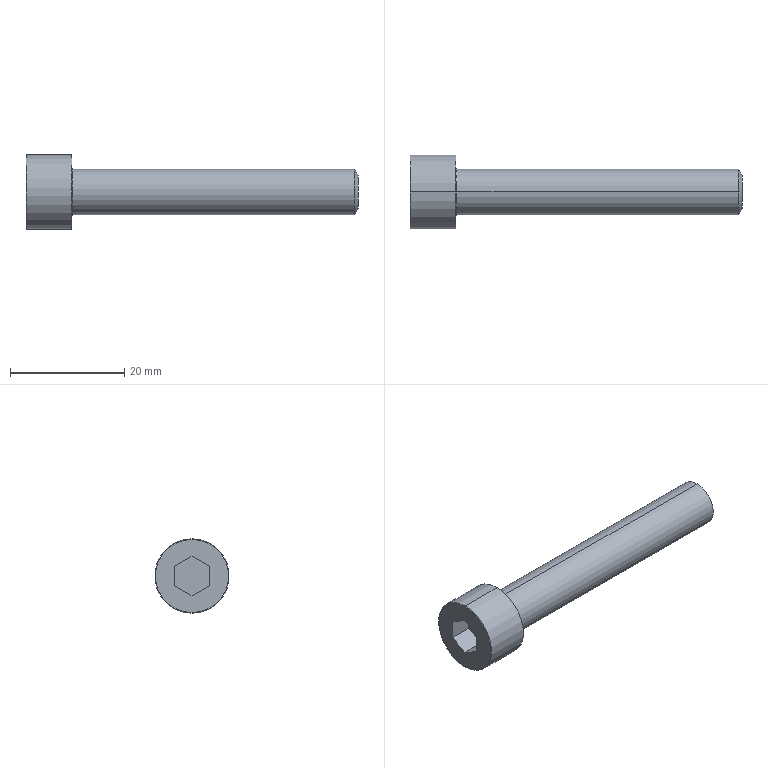Part | STEP file | 1 solid | 20 faces | box 58 x 13 x 13 mm | volume 3445 mm3 | plane 10 | torus 4 | cylinder 4 | cone 2 | commonest cylinder face diameters 8 x2 13 x2
STEP:
#1=CARTESIAN_POINT('',(0.,0.,0.));
#2=DIRECTION('',(0.,0.,1.));
#3=DIRECTION('',(1.,0.,0.));
#4=AXIS2_PLACEMENT_3D('',#1,#2,#3);
#5=CARTESIAN_POINT('',(0.,0.,6.4));
#6=VERTEX_POINT('',#5);
#7=CARTESIAN_POINT('',(0.1,0.,6.5));
#8=VERTEX_POINT('',#7);
#9=CARTESIAN_POINT('',(0.1,0.,6.4));
#10=DIRECTION('',(0.,1.,0.));
#11=DIRECTION('',(0.,0.,1.));
#12=AXIS2_PLACEMENT_3D('',#9,#10,#11);
#13=CIRCLE('',#12,0.1);
#14=CARTESIAN_POINT('',(0.1,0.,0.));
#15=DIRECTION('',(1.,0.,0.));
#16=DIRECTION('',(0.,0.,-1.));
#17=AXIS2_PLACEMENT_3D('',#14,#15,#16);
#18=TOROIDAL_SURFACE('',#17,6.4,0.1);
#19=CARTESIAN_POINT('',(3.142,0.));
#20=DIRECTION('',(0.,1.));
#21=VECTOR('',#20,1.);
#22=LINE('',#19,#21);
#23=(GEOMETRIC_REPRESENTATION_CONTEXT(2)PARAMETRIC_REPRESENTATION_CONTEXT()REPRESENTATION_CONTEXT('',''));
#24=DEFINITIONAL_REPRESENTATION('',(#22),#23);
#25=PCURVE('',#18,#24);
#26=CARTESIAN_POINT('',(0.1,0.,0.));
#27=DIRECTION('',(1.,0.,0.));
#28=DIRECTION('',(0.,0.,-1.));
#29=AXIS2_PLACEMENT_3D('',#26,#27,#28);
#30=TOROIDAL_SURFACE('',#29,6.4,0.1);
#31=CARTESIAN_POINT('',(3.142,0.));
#32=DIRECTION('',(0.,1.));
#33=VECTOR('',#32,1.);
#34=LINE('',#31,#33);
#35=(GEOMETRIC_REPRESENTATION_CONTEXT(2)PARAMETRIC_REPRESENTATION_CONTEXT()REPRESENTATION_CONTEXT('',''));
#36=DEFINITIONAL_REPRESENTATION('',(#34),#35);
#37=PCURVE('',#30,#36);
#38=SURFACE_CURVE('',#13,(#25,#37),.PCURVE_S1.);
#39=EDGE_CURVE('',#6,#8,#38,.T.);
#40=ORIENTED_EDGE('',*,*,#39,.F.);
#41=CARTESIAN_POINT('',(0.,0.,-6.4));
#42=VERTEX_POINT('',#41);
#43=CARTESIAN_POINT('',(0.,0.,0.));
#44=DIRECTION('',(-1.,0.,0.));
#45=DIRECTION('',(0.,0.,-1.));
#46=AXIS2_PLACEMENT_3D('',#43,#44,#45);
#47=CIRCLE('',#46,6.4);
#48=CARTESIAN_POINT('',(6.283,4.712));
#49=DIRECTION('',(-1.,0.));
#50=VECTOR('',#49,1.);
#51=LINE('',#48,#50);
#52=(GEOMETRIC_REPRESENTATION_CONTEXT(2)PARAMETRIC_REPRESENTATION_CONTEXT()REPRESENTATION_CONTEXT('',''));
#53=DEFINITIONAL_REPRESENTATION('',(#51),#52);
#54=PCURVE('',#18,#53);
#55=CARTESIAN_POINT('',(0.,0.,0.));
#56=DIRECTION('',(1.,0.,0.));
#57=DIRECTION('',(0.,0.,-1.));
#58=AXIS2_PLACEMENT_3D('',#55,#56,#57);
#59=PLANE('',#58);
#60=CARTESIAN_POINT('',(6.4,0.));
#61=CARTESIAN_POINT('',(6.4,-11.085));
#62=CARTESIAN_POINT('',(-3.2,-5.543));
#63=CARTESIAN_POINT('',(-12.8,0.));
#64=CARTESIAN_POINT('',(-3.2,5.543));
#65=CARTESIAN_POINT('',(6.4,11.085));
#66=CARTESIAN_POINT('',(6.4,0.));
#67=(BOUNDED_CURVE()B_SPLINE_CURVE(2,(#60,#61,#62,#63,#64,#65,#66),.UNSPECIFIED.,.T.,.F.)B_SPLINE_CURVE_WITH_KNOTS((1,2,2,2,2,1),(-2.094,0.,2.094,4.189,6.283,8.378),.UNSPECIFIED.)CURVE()GEOMETRIC_REPRESENTATION_ITEM()RATIONAL_B_SPLINE_CURVE((1.,0.5,1.,0.5,1.,0.5,1.))REPRESENTATION_ITEM(''));
#68=(GEOMETRIC_REPRESENTATION_CONTEXT(2)PARAMETRIC_REPRESENTATION_CONTEXT()REPRESENTATION_CONTEXT('',''));
#69=DEFINITIONAL_REPRESENTATION('',(#67),#68);
#70=PCURVE('',#59,#69);
#71=SURFACE_CURVE('',#47,(#54,#70),.PCURVE_S1.);
#72=EDGE_CURVE('',#42,#6,#71,.T.);
#73=ORIENTED_EDGE('',*,*,#72,.F.);
#74=CARTESIAN_POINT('',(0.1,0.,-6.5));
#75=VERTEX_POINT('',#74);
#76=CARTESIAN_POINT('',(0.1,0.,-6.4));
#77=DIRECTION('',(0.,-1.,0.));
#78=DIRECTION('',(0.,0.,-1.));
#79=AXIS2_PLACEMENT_3D('',#76,#77,#78);
#80=CIRCLE('',#79,0.1);
#81=CARTESIAN_POINT('',(6.283,0.));
#82=DIRECTION('',(0.,1.));
#83=VECTOR('',#82,1.);
#84=LINE('',#81,#83);
#85=(GEOMETRIC_REPRESENTATION_CONTEXT(2)PARAMETRIC_REPRESENTATION_CONTEXT()REPRESENTATION_CONTEXT('',''));
#86=DEFINITIONAL_REPRESENTATION('',(#84),#85);
#87=PCURVE('',#18,#86);
#88=CARTESIAN_POINT('',(0.,0.));
#89=DIRECTION('',(0.,1.));
#90=VECTOR('',#89,1.);
#91=LINE('',#88,#90);
#92=(GEOMETRIC_REPRESENTATION_CONTEXT(2)PARAMETRIC_REPRESENTATION_CONTEXT()REPRESENTATION_CONTEXT('',''));
#93=DEFINITIONAL_REPRESENTATION('',(#91),#92);
#94=PCURVE('',#30,#93);
#95=SURFACE_CURVE('',#80,(#87,#94),.PCURVE_S1.);
#96=EDGE_CURVE('',#42,#75,#95,.T.);
#97=ORIENTED_EDGE('',*,*,#96,.T.);
#98=CARTESIAN_POINT('',(0.1,0.,0.));
#99=DIRECTION('',(1.,0.,0.));
#100=DIRECTION('',(0.,0.,-1.));
#101=AXIS2_PLACEMENT_3D('',#98,#99,#100);
#102=CIRCLE('',#101,6.5);
#103=CARTESIAN_POINT('',(0.,6.283));
#104=DIRECTION('',(1.,0.));
#105=VECTOR('',#104,1.);
#106=LINE('',#103,#105);
#107=(GEOMETRIC_REPRESENTATION_CONTEXT(2)PARAMETRIC_REPRESENTATION_CONTEXT()REPRESENTATION_CONTEXT('',''));
#108=DEFINITIONAL_REPRESENTATION('',(#106),#107);
#109=PCURVE('',#18,#108);
#110=CARTESIAN_POINT('',(0.,0.,0.));
#111=DIRECTION('',(-1.,0.,0.));
#112=DIRECTION('',(0.,0.,1.));
#113=AXIS2_PLACEMENT_3D('',#110,#111,#112);
#114=CYLINDRICAL_SURFACE('',#113,6.5);
#115=CARTESIAN_POINT('',(9.425,-0.1));
#116=DIRECTION('',(-1.,0.));
#117=VECTOR('',#116,1.);
#118=LINE('',#115,#117);
#119=(GEOMETRIC_REPRESENTATION_CONTEXT(2)PARAMETRIC_REPRESENTATION_CONTEXT()REPRESENTATION_CONTEXT('',''));
#120=DEFINITIONAL_REPRESENTATION('',(#118),#119);
#121=PCURVE('',#114,#120);
#122=SURFACE_CURVE('',#102,(#109,#121),.PCURVE_S1.);
#123=EDGE_CURVE('',#8,#75,#122,.T.);
#124=ORIENTED_EDGE('',*,*,#123,.F.);
#125=EDGE_LOOP('',(#40,#73,#97,#124));
#126=FACE_BOUND('',#125,.T.);
#127=ADVANCED_FACE('',(#126),#18,.T.);
#128=CARTESIAN_POINT('',(58.,0.,2.917));
#129=VERTEX_POINT('',#128);
#130=CARTESIAN_POINT('',(58.,0.,-2.917));
#131=VERTEX_POINT('',#130);
#132=CARTESIAN_POINT('',(58.,0.,0.));
#133=DIRECTION('',(-1.,0.,0.));
#134=DIRECTION('',(0.,0.,1.));
#135=AXIS2_PLACEMENT_3D('',#132,#133,#134);
#136=CIRCLE('',#135,2.917);
#137=CARTESIAN_POINT('',(58.,4.,0.));
#138=DIRECTION('',(-1.,0.,0.));
#139=DIRECTION('',(0.,0.,1.));
#140=AXIS2_PLACEMENT_3D('',#137,#138,#139);
#141=PLANE('',#140);
#142=CARTESIAN_POINT('',(0.,-4.));
#143=DIRECTION('',(1.,0.));
#144=AXIS2_PLACEMENT_2D('',#142,#143);
#145=CIRCLE('',#144,2.917);
#146=(GEOMETRIC_REPRESENTATION_CONTEXT(2)PARAMETRIC_REPRESENTATION_CONTEXT()REPRESENTATION_CONTEXT('',''));
#147=DEFINITIONAL_REPRESENTATION('',(#145),#146);
#148=PCURVE('',#141,#147);
#149=CARTESIAN_POINT('',(57.375,0.,0.));
#150=DIRECTION('',(-1.,0.,0.));
#151=DIRECTION('',(0.,0.,1.));
#152=AXIS2_PLACEMENT_3D('',#149,#150,#151);
#153=CONICAL_SURFACE('',#152,4.,1.047);
#154=CARTESIAN_POINT('',(0.,-0.625));
#155=DIRECTION('',(1.,0.));
#156=VECTOR('',#155,1.);
#157=LINE('',#154,#156);
#158=(GEOMETRIC_REPRESENTATION_CONTEXT(2)PARAMETRIC_REPRESENTATION_CONTEXT()REPRESENTATION_CONTEXT('',''));
#159=DEFINITIONAL_REPRESENTATION('',(#157),#158);
#160=PCURVE('',#153,#159);
#161=SURFACE_CURVE('',#136,(#148,#160),.PCURVE_S1.);
#162=EDGE_CURVE('',#129,#131,#161,.T.);
#163=ORIENTED_EDGE('',*,*,#162,.F.);
#164=CARTESIAN_POINT('',(58.,0.,0.));
#165=DIRECTION('',(-1.,0.,0.));
#166=DIRECTION('',(0.,0.,1.));
#167=AXIS2_PLACEMENT_3D('',#164,#165,#166);
#168=CIRCLE('',#167,2.917);
#169=CARTESIAN_POINT('',(0.,-4.));
#170=DIRECTION('',(1.,0.));
#171=AXIS2_PLACEMENT_2D('',#169,#170);
#172=CIRCLE('',#171,2.917);
#173=(GEOMETRIC_REPRESENTATION_CONTEXT(2)PARAMETRIC_REPRESENTATION_CONTEXT()REPRESENTATION_CONTEXT('',''));
#174=DEFINITIONAL_REPRESENTATION('',(#172),#173);
#175=PCURVE('',#141,#174);
#176=CARTESIAN_POINT('',(57.375,0.,0.));
#177=DIRECTION('',(-1.,0.,0.));
#178=DIRECTION('',(0.,0.,1.));
#179=AXIS2_PLACEMENT_3D('',#176,#177,#178);
#180=CONICAL_SURFACE('',#179,4.,1.047);
#181=CARTESIAN_POINT('',(0.,-0.625));
#182=DIRECTION('',(1.,0.));
#183=VECTOR('',#182,1.);
#184=LINE('',#181,#183);
#185=(GEOMETRIC_REPRESENTATION_CONTEXT(2)PARAMETRIC_REPRESENTATION_CONTEXT()REPRESENTATION_CONTEXT('',''));
#186=DEFINITIONAL_REPRESENTATION('',(#184),#185);
#187=PCURVE('',#180,#186);
#188=SURFACE_CURVE('',#168,(#175,#187),.PCURVE_S1.);
#189=EDGE_CURVE('',#131,#129,#188,.T.);
#190=ORIENTED_EDGE('',*,*,#189,.F.);
#191=EDGE_LOOP('',(#163,#190));
#192=FACE_BOUND('',#191,.T.);
#193=ADVANCED_FACE('',(#192),#141,.F.);
#194=CARTESIAN_POINT('',(57.375,0.,-4.));
#195=VERTEX_POINT('',#194);
#196=CARTESIAN_POINT('',(57.375,0.,-4.));
#197=DIRECTION('',(-0.5,0.,-0.866));
#198=VECTOR('',#197,1.);
#199=LINE('',#196,#198);
#200=CARTESIAN_POINT('',(3.142,0.));
#201=DIRECTION('',(0.,1.));
#202=VECTOR('',#201,1.);
#203=LINE('',#200,#202);
#204=(GEOMETRIC_REPRESENTATION_CONTEXT(2)PARAMETRIC_REPRESENTATION_CONTEXT()REPRESENTATION_CONTEXT('',''));
#205=DEFINITIONAL_REPRESENTATION('',(#203),#204);
#206=PCURVE('',#180,#205);
#207=CARTESIAN_POINT('',(3.142,0.));
#208=DIRECTION('',(0.,1.));
#209=VECTOR('',#208,1.);
#210=LINE('',#207,#209);
#211=(GEOMETRIC_REPRESENTATION_CONTEXT(2)PARAMETRIC_REPRESENTATION_CONTEXT()REPRESENTATION_CONTEXT('',''));
#212=DEFINITIONAL_REPRESENTATION('',(#210),#211);
#213=PCURVE('',#153,#212);
#214=SURFACE_CURVE('',#199,(#206,#213),.PCURVE_S1.);
#215=EDGE_CURVE('',#131,#195,#214,.T.);
#216=ORIENTED_EDGE('',*,*,#215,.F.);
#217=ORIENTED_EDGE('',*,*,#189,.T.);
#218=CARTESIAN_POINT('',(57.375,0.,4.));
#219=VERTEX_POINT('',#218);
#220=CARTESIAN_POINT('',(57.375,0.,4.));
#221=DIRECTION('',(-0.5,0.,0.866));
#222=VECTOR('',#221,1.);
#223=LINE('',#220,#222);
#224=CARTESIAN_POINT('',(6.283,0.));
#225=DIRECTION('',(0.,1.));
#226=VECTOR('',#225,1.);
#227=LINE('',#224,#226);
#228=(GEOMETRIC_REPRESENTATION_CONTEXT(2)PARAMETRIC_REPRESENTATION_CONTEXT()REPRESENTATION_CONTEXT('',''));
#229=DEFINITIONAL_REPRESENTATION('',(#227),#228);
#230=PCURVE('',#180,#229);
#231=CARTESIAN_POINT('',(0.,0.));
#232=DIRECTION('',(0.,1.));
#233=VECTOR('',#232,1.);
#234=LINE('',#231,#233);
#235=(GEOMETRIC_REPRESENTATION_CONTEXT(2)PARAMETRIC_REPRESENTATION_CONTEXT()REPRESENTATION_CONTEXT('',''));
#236=DEFINITIONAL_REPRESENTATION('',(#234),#235);
#237=PCURVE('',#153,#236);
#238=SURFACE_CURVE('',#223,(#230,#237),.PCURVE_S1.);
#239=EDGE_CURVE('',#129,#219,#238,.T.);
#240=ORIENTED_EDGE('',*,*,#239,.T.);
#241=CARTESIAN_POINT('',(57.375,0.,0.));
#242=DIRECTION('',(-1.,0.,0.));
#243=DIRECTION('',(0.,0.,1.));
#244=AXIS2_PLACEMENT_3D('',#241,#242,#243);
#245=CIRCLE('',#244,4.);
#246=CARTESIAN_POINT('',(0.,0.));
#247=DIRECTION('',(1.,0.));
#248=VECTOR('',#247,1.);
#249=LINE('',#246,#248);
#250=(GEOMETRIC_REPRESENTATION_CONTEXT(2)PARAMETRIC_REPRESENTATION_CONTEXT()REPRESENTATION_CONTEXT('',''));
#251=DEFINITIONAL_REPRESENTATION('',(#249),#250);
#252=PCURVE('',#180,#251);
#253=CARTESIAN_POINT('',(0.,0.,0.));
#254=DIRECTION('',(-1.,0.,0.));
#255=DIRECTION('',(0.,0.,1.));
#256=AXIS2_PLACEMENT_3D('',#253,#254,#255);
#257=CYLINDRICAL_SURFACE('',#256,4.);
#258=CARTESIAN_POINT('',(0.,-57.375));
#259=DIRECTION('',(1.,0.));
#260=VECTOR('',#259,1.);
#261=LINE('',#258,#260);
#262=(GEOMETRIC_REPRESENTATION_CONTEXT(2)PARAMETRIC_REPRESENTATION_CONTEXT()REPRESENTATION_CONTEXT('',''));
#263=DEFINITIONAL_REPRESENTATION('',(#261),#262);
#264=PCURVE('',#257,#263);
#265=SURFACE_CURVE('',#245,(#252,#264),.PCURVE_S1.);
#266=EDGE_CURVE('',#195,#219,#265,.T.);
#267=ORIENTED_EDGE('',*,*,#266,.F.);
#268=EDGE_LOOP('',(#216,#217,#240,#267));
#269=FACE_BOUND('',#268,.T.);
#270=ADVANCED_FACE('',(#269),#180,.T.);
#271=CARTESIAN_POINT('',(4.,-2.97,1.715));
#272=VERTEX_POINT('',#271);
#273=CARTESIAN_POINT('',(4.,0.,3.43));
#274=VERTEX_POINT('',#273);
#275=CARTESIAN_POINT('',(4.,-2.97,1.715));
#276=DIRECTION('',(0.,0.866,0.5));
#277=VECTOR('',#276,1.);
#278=LINE('',#275,#277);
#279=CARTESIAN_POINT('',(4.,-2.97,1.715));
#280=DIRECTION('',(1.,0.,0.));
#281=DIRECTION('',(0.,0.,-1.));
#282=AXIS2_PLACEMENT_3D('',#279,#280,#281);
#283=PLANE('',#282);
#284=CARTESIAN_POINT('',(0.,0.));
#285=DIRECTION('',(-0.5,0.866));
#286=VECTOR('',#285,1.);
#287=LINE('',#284,#286);
#288=(GEOMETRIC_REPRESENTATION_CONTEXT(2)PARAMETRIC_REPRESENTATION_CONTEXT()REPRESENTATION_CONTEXT('',''));
#289=DEFINITIONAL_REPRESENTATION('',(#287),#288);
#290=PCURVE('',#283,#289);
#291=CARTESIAN_POINT('',(4.,-2.97,1.715));
#292=DIRECTION('',(0.,-0.5,0.866));
#293=DIRECTION('',(0.,-0.866,-0.5));
#294=AXIS2_PLACEMENT_3D('',#291,#292,#293);
#295=PLANE('',#294);
#296=CARTESIAN_POINT('',(0.,0.));
#297=DIRECTION('',(-1.,0.));
#298=VECTOR('',#297,1.);
#299=LINE('',#296,#298);
#300=(GEOMETRIC_REPRESENTATION_CONTEXT(2)PARAMETRIC_REPRESENTATION_CONTEXT()REPRESENTATION_CONTEXT('',''));
#301=DEFINITIONAL_REPRESENTATION('',(#299),#300);
#302=PCURVE('',#295,#301);
#303=SURFACE_CURVE('',#278,(#290,#302),.PCURVE_S1.);
#304=EDGE_CURVE('',#272,#274,#303,.T.);
#305=ORIENTED_EDGE('',*,*,#304,.T.);
#306=CARTESIAN_POINT('',(4.,2.97,1.715));
#307=VERTEX_POINT('',#306);
#308=CARTESIAN_POINT('',(4.,0.,3.43));
#309=DIRECTION('',(0.,0.866,-0.5));
#310=VECTOR('',#309,1.);
#311=LINE('',#308,#310);
#312=CARTESIAN_POINT('',(-1.715,2.97));
#313=DIRECTION('',(0.5,0.866));
#314=VECTOR('',#313,1.);
#315=LINE('',#312,#314);
#316=(GEOMETRIC_REPRESENTATION_CONTEXT(2)PARAMETRIC_REPRESENTATION_CONTEXT()REPRESENTATION_CONTEXT('',''));
#317=DEFINITIONAL_REPRESENTATION('',(#315),#316);
#318=PCURVE('',#283,#317);
#319=CARTESIAN_POINT('',(4.,0.,3.43));
#320=DIRECTION('',(0.,0.5,0.866));
#321=DIRECTION('',(0.,-0.866,0.5));
#322=AXIS2_PLACEMENT_3D('',#319,#320,#321);
#323=PLANE('',#322);
#324=CARTESIAN_POINT('',(0.,0.));
#325=DIRECTION('',(-1.,0.));
#326=VECTOR('',#325,1.);
#327=LINE('',#324,#326);
#328=(GEOMETRIC_REPRESENTATION_CONTEXT(2)PARAMETRIC_REPRESENTATION_CONTEXT()REPRESENTATION_CONTEXT('',''));
#329=DEFINITIONAL_REPRESENTATION('',(#327),#328);
#330=PCURVE('',#323,#329);
#331=SURFACE_CURVE('',#311,(#318,#330),.PCURVE_S1.);
#332=EDGE_CURVE('',#274,#307,#331,.T.);
#333=ORIENTED_EDGE('',*,*,#332,.T.);
#334=CARTESIAN_POINT('',(4.,2.97,-1.715));
#335=VERTEX_POINT('',#334);
#336=CARTESIAN_POINT('',(4.,2.97,1.715));
#337=DIRECTION('',(0.,0.,-1.));
#338=VECTOR('',#337,1.);
#339=LINE('',#336,#338);
#340=CARTESIAN_POINT('',(0.,5.941));
#341=DIRECTION('',(1.,0.));
#342=VECTOR('',#341,1.);
#343=LINE('',#340,#342);
#344=(GEOMETRIC_REPRESENTATION_CONTEXT(2)PARAMETRIC_REPRESENTATION_CONTEXT()REPRESENTATION_CONTEXT('',''));
#345=DEFINITIONAL_REPRESENTATION('',(#343),#344);
#346=PCURVE('',#283,#345);
#347=CARTESIAN_POINT('',(4.,2.97,1.715));
#348=DIRECTION('',(0.,1.,0.));
#349=DIRECTION('',(0.,0.,1.));
#350=AXIS2_PLACEMENT_3D('',#347,#348,#349);
#351=PLANE('',#350);
#352=CARTESIAN_POINT('',(0.,0.));
#353=DIRECTION('',(-1.,0.));
#354=VECTOR('',#353,1.);
#355=LINE('',#352,#354);
#356=(GEOMETRIC_REPRESENTATION_CONTEXT(2)PARAMETRIC_REPRESENTATION_CONTEXT()REPRESENTATION_CONTEXT('',''));
#357=DEFINITIONAL_REPRESENTATION('',(#355),#356);
#358=PCURVE('',#351,#357);
#359=SURFACE_CURVE('',#339,(#346,#358),.PCURVE_S1.);
#360=EDGE_CURVE('',#307,#335,#359,.T.);
#361=ORIENTED_EDGE('',*,*,#360,.T.);
#362=CARTESIAN_POINT('',(4.,0.,-3.43));
#363=VERTEX_POINT('',#362);
#364=CARTESIAN_POINT('',(4.,2.97,-1.715));
#365=DIRECTION('',(0.,-0.866,-0.5));
#366=VECTOR('',#365,1.);
#367=LINE('',#364,#366);
#368=CARTESIAN_POINT('',(3.43,5.941));
#369=DIRECTION('',(0.5,-0.866));
#370=VECTOR('',#369,1.);
#371=LINE('',#368,#370);
#372=(GEOMETRIC_REPRESENTATION_CONTEXT(2)PARAMETRIC_REPRESENTATION_CONTEXT()REPRESENTATION_CONTEXT('',''));
#373=DEFINITIONAL_REPRESENTATION('',(#371),#372);
#374=PCURVE('',#283,#373);
#375=CARTESIAN_POINT('',(4.,2.97,-1.715));
#376=DIRECTION('',(0.,0.5,-0.866));
#377=DIRECTION('',(0.,0.866,0.5));
#378=AXIS2_PLACEMENT_3D('',#375,#376,#377);
#379=PLANE('',#378);
#380=CARTESIAN_POINT('',(0.,0.));
#381=DIRECTION('',(-1.,0.));
#382=VECTOR('',#381,1.);
#383=LINE('',#380,#382);
#384=(GEOMETRIC_REPRESENTATION_CONTEXT(2)PARAMETRIC_REPRESENTATION_CONTEXT()REPRESENTATION_CONTEXT('',''));
#385=DEFINITIONAL_REPRESENTATION('',(#383),#384);
#386=PCURVE('',#379,#385);
#387=SURFACE_CURVE('',#367,(#374,#386),.PCURVE_S1.);
#388=EDGE_CURVE('',#335,#363,#387,.T.);
#389=ORIENTED_EDGE('',*,*,#388,.T.);
#390=CARTESIAN_POINT('',(4.,-2.97,-1.715));
#391=VERTEX_POINT('',#390);
#392=CARTESIAN_POINT('',(4.,0.,-3.43));
#393=DIRECTION('',(0.,-0.866,0.5));
#394=VECTOR('',#393,1.);
#395=LINE('',#392,#394);
#396=CARTESIAN_POINT('',(5.145,2.97));
#397=DIRECTION('',(-0.5,-0.866));
#398=VECTOR('',#397,1.);
#399=LINE('',#396,#398);
#400=(GEOMETRIC_REPRESENTATION_CONTEXT(2)PARAMETRIC_REPRESENTATION_CONTEXT()REPRESENTATION_CONTEXT('',''));
#401=DEFINITIONAL_REPRESENTATION('',(#399),#400);
#402=PCURVE('',#283,#401);
#403=CARTESIAN_POINT('',(4.,0.,-3.43));
#404=DIRECTION('',(0.,-0.5,-0.866));
#405=DIRECTION('',(0.,0.866,-0.5));
#406=AXIS2_PLACEMENT_3D('',#403,#404,#405);
#407=PLANE('',#406);
#408=CARTESIAN_POINT('',(0.,0.));
#409=DIRECTION('',(-1.,0.));
#410=VECTOR('',#409,1.);
#411=LINE('',#408,#410);
#412=(GEOMETRIC_REPRESENTATION_CONTEXT(2)PARAMETRIC_REPRESENTATION_CONTEXT()REPRESENTATION_CONTEXT('',''));
#413=DEFINITIONAL_REPRESENTATION('',(#411),#412);
#414=PCURVE('',#407,#413);
#415=SURFACE_CURVE('',#395,(#402,#414),.PCURVE_S1.);
#416=EDGE_CURVE('',#363,#391,#415,.T.);
#417=ORIENTED_EDGE('',*,*,#416,.T.);
#418=CARTESIAN_POINT('',(4.,-2.97,-1.715));
#419=DIRECTION('',(0.,0.,1.));
#420=VECTOR('',#419,1.);
#421=LINE('',#418,#420);
#422=CARTESIAN_POINT('',(3.43,0.));
#423=DIRECTION('',(-1.,0.));
#424=VECTOR('',#423,1.);
#425=LINE('',#422,#424);
#426=(GEOMETRIC_REPRESENTATION_CONTEXT(2)PARAMETRIC_REPRESENTATION_CONTEXT()REPRESENTATION_CONTEXT('',''));
#427=DEFINITIONAL_REPRESENTATION('',(#425),#426);
#428=PCURVE('',#283,#427);
#429=CARTESIAN_POINT('',(4.,-2.97,-1.715));
#430=DIRECTION('',(0.,-1.,0.));
#431=DIRECTION('',(0.,0.,-1.));
#432=AXIS2_PLACEMENT_3D('',#429,#430,#431);
#433=PLANE('',#432);
#434=CARTESIAN_POINT('',(0.,0.));
#435=DIRECTION('',(-1.,0.));
#436=VECTOR('',#435,1.);
#437=LINE('',#434,#436);
#438=(GEOMETRIC_REPRESENTATION_CONTEXT(2)PARAMETRIC_REPRESENTATION_CONTEXT()REPRESENTATION_CONTEXT('',''));
#439=DEFINITIONAL_REPRESENTATION('',(#437),#438);
#440=PCURVE('',#433,#439);
#441=SURFACE_CURVE('',#421,(#428,#440),.PCURVE_S1.);
#442=EDGE_CURVE('',#391,#272,#441,.T.);
#443=ORIENTED_EDGE('',*,*,#442,.T.);
#444=EDGE_LOOP('',(#305,#333,#361,#389,#417,#443));
#445=FACE_BOUND('',#444,.T.);
#446=ADVANCED_FACE('',(#445),#283,.F.);
#447=CARTESIAN_POINT('',(0.,0.,3.43));
#448=VERTEX_POINT('',#447);
#449=CARTESIAN_POINT('',(0.,2.97,1.715));
#450=VERTEX_POINT('',#449);
#451=CARTESIAN_POINT('',(0.,0.,3.43));
#452=DIRECTION('',(0.,0.866,-0.5));
#453=VECTOR('',#452,1.);
#454=LINE('',#451,#453);
#455=CARTESIAN_POINT('',(0.,-4.));
#456=DIRECTION('',(-1.,0.));
#457=VECTOR('',#456,1.);
#458=LINE('',#455,#457);
#459=(GEOMETRIC_REPRESENTATION_CONTEXT(2)PARAMETRIC_REPRESENTATION_CONTEXT()REPRESENTATION_CONTEXT('',''));
#460=DEFINITIONAL_REPRESENTATION('',(#458),#459);
#461=PCURVE('',#323,#460);
#462=CARTESIAN_POINT('',(-3.43,0.));
#463=DIRECTION('',(0.5,0.866));
#464=VECTOR('',#463,1.);
#465=LINE('',#462,#464);
#466=(GEOMETRIC_REPRESENTATION_CONTEXT(2)PARAMETRIC_REPRESENTATION_CONTEXT()REPRESENTATION_CONTEXT('',''));
#467=DEFINITIONAL_REPRESENTATION('',(#465),#466);
#468=PCURVE('',#59,#467);
#469=SURFACE_CURVE('',#454,(#461,#468),.PCURVE_S1.);
#470=EDGE_CURVE('',#448,#450,#469,.T.);
#471=ORIENTED_EDGE('',*,*,#470,.T.);
#472=CARTESIAN_POINT('',(4.,2.97,1.715));
#473=DIRECTION('',(-1.,0.,0.));
#474=VECTOR('',#473,1.);
#475=LINE('',#472,#474);
#476=CARTESIAN_POINT('',(-3.43,0.));
#477=DIRECTION('',(0.,-1.));
#478=VECTOR('',#477,1.);
#479=LINE('',#476,#478);
#480=(GEOMETRIC_REPRESENTATION_CONTEXT(2)PARAMETRIC_REPRESENTATION_CONTEXT()REPRESENTATION_CONTEXT('',''));
#481=DEFINITIONAL_REPRESENTATION('',(#479),#480);
#482=PCURVE('',#323,#481);
#483=CARTESIAN_POINT('',(0.,0.));
#484=DIRECTION('',(0.,-1.));
#485=VECTOR('',#484,1.);
#486=LINE('',#483,#485);
#487=(GEOMETRIC_REPRESENTATION_CONTEXT(2)PARAMETRIC_REPRESENTATION_CONTEXT()REPRESENTATION_CONTEXT('',''));
#488=DEFINITIONAL_REPRESENTATION('',(#486),#487);
#489=PCURVE('',#351,#488);
#490=SURFACE_CURVE('',#475,(#482,#489),.PCURVE_S1.);
#491=EDGE_CURVE('',#307,#450,#490,.T.);
#492=ORIENTED_EDGE('',*,*,#491,.F.);
#493=ORIENTED_EDGE('',*,*,#332,.F.);
#494=CARTESIAN_POINT('',(4.,0.,3.43));
#495=DIRECTION('',(-1.,0.,0.));
#496=VECTOR('',#495,1.);
#497=LINE('',#494,#496);
#498=CARTESIAN_POINT('',(0.,0.));
#499=DIRECTION('',(0.,-1.));
#500=VECTOR('',#499,1.);
#501=LINE('',#498,#500);
#502=(GEOMETRIC_REPRESENTATION_CONTEXT(2)PARAMETRIC_REPRESENTATION_CONTEXT()REPRESENTATION_CONTEXT('',''));
#503=DEFINITIONAL_REPRESENTATION('',(#501),#502);
#504=PCURVE('',#323,#503);
#505=CARTESIAN_POINT('',(-3.43,0.));
#506=DIRECTION('',(0.,-1.));
#507=VECTOR('',#506,1.);
#508=LINE('',#505,#507);
#509=(GEOMETRIC_REPRESENTATION_CONTEXT(2)PARAMETRIC_REPRESENTATION_CONTEXT()REPRESENTATION_CONTEXT('',''));
#510=DEFINITIONAL_REPRESENTATION('',(#508),#509);
#511=PCURVE('',#295,#510);
#512=SURFACE_CURVE('',#497,(#504,#511),.PCURVE_S1.);
#513=EDGE_CURVE('',#274,#448,#512,.T.);
#514=ORIENTED_EDGE('',*,*,#513,.T.);
#515=EDGE_LOOP('',(#471,#492,#493,#514));
#516=FACE_BOUND('',#515,.T.);
#517=ADVANCED_FACE('',(#516),#323,.F.);
#518=CARTESIAN_POINT('',(0.,2.97,-1.715));
#519=VERTEX_POINT('',#518);
#520=CARTESIAN_POINT('',(0.,2.97,1.715));
#521=DIRECTION('',(0.,0.,-1.));
#522=VECTOR('',#521,1.);
#523=LINE('',#520,#522);
#524=CARTESIAN_POINT('',(0.,-4.));
#525=DIRECTION('',(-1.,0.));
#526=VECTOR('',#525,1.);
#527=LINE('',#524,#526);
#528=(GEOMETRIC_REPRESENTATION_CONTEXT(2)PARAMETRIC_REPRESENTATION_CONTEXT()REPRESENTATION_CONTEXT('',''));
#529=DEFINITIONAL_REPRESENTATION('',(#527),#528);
#530=PCURVE('',#351,#529);
#531=CARTESIAN_POINT('',(-1.715,2.97));
#532=DIRECTION('',(1.,0.));
#533=VECTOR('',#532,1.);
#534=LINE('',#531,#533);
#535=(GEOMETRIC_REPRESENTATION_CONTEXT(2)PARAMETRIC_REPRESENTATION_CONTEXT()REPRESENTATION_CONTEXT('',''));
#536=DEFINITIONAL_REPRESENTATION('',(#534),#535);
#537=PCURVE('',#59,#536);
#538=SURFACE_CURVE('',#523,(#530,#537),.PCURVE_S1.);
#539=EDGE_CURVE('',#450,#519,#538,.T.);
#540=ORIENTED_EDGE('',*,*,#539,.T.);
#541=CARTESIAN_POINT('',(4.,2.97,-1.715));
#542=DIRECTION('',(-1.,0.,0.));
#543=VECTOR('',#542,1.);
#544=LINE('',#541,#543);
#545=CARTESIAN_POINT('',(-3.43,0.));
#546=DIRECTION('',(0.,-1.));
#547=VECTOR('',#546,1.);
#548=LINE('',#545,#547);
#549=(GEOMETRIC_REPRESENTATION_CONTEXT(2)PARAMETRIC_REPRESENTATION_CONTEXT()REPRESENTATION_CONTEXT('',''));
#550=DEFINITIONAL_REPRESENTATION('',(#548),#549);
#551=PCURVE('',#351,#550);
#552=CARTESIAN_POINT('',(0.,0.));
#553=DIRECTION('',(0.,-1.));
#554=VECTOR('',#553,1.);
#555=LINE('',#552,#554);
#556=(GEOMETRIC_REPRESENTATION_CONTEXT(2)PARAMETRIC_REPRESENTATION_CONTEXT()REPRESENTATION_CONTEXT('',''));
#557=DEFINITIONAL_REPRESENTATION('',(#555),#556);
#558=PCURVE('',#379,#557);
#559=SURFACE_CURVE('',#544,(#551,#558),.PCURVE_S1.);
#560=EDGE_CURVE('',#335,#519,#559,.T.);
#561=ORIENTED_EDGE('',*,*,#560,.F.);
#562=ORIENTED_EDGE('',*,*,#360,.F.);
#563=ORIENTED_EDGE('',*,*,#491,.T.);
#564=EDGE_LOOP('',(#540,#561,#562,#563));
#565=FACE_BOUND('',#564,.T.);
#566=ADVANCED_FACE('',(#565),#351,.F.);
#567=CARTESIAN_POINT('',(0.,0.,-3.43));
#568=VERTEX_POINT('',#567);
#569=CARTESIAN_POINT('',(0.,2.97,-1.715));
#570=DIRECTION('',(0.,-0.866,-0.5));
#571=VECTOR('',#570,1.);
#572=LINE('',#569,#571);
#573=CARTESIAN_POINT('',(0.,-4.));
#574=DIRECTION('',(-1.,0.));
#575=VECTOR('',#574,1.);
#576=LINE('',#573,#575);
#577=(GEOMETRIC_REPRESENTATION_CONTEXT(2)PARAMETRIC_REPRESENTATION_CONTEXT()REPRESENTATION_CONTEXT('',''));
#578=DEFINITIONAL_REPRESENTATION('',(#576),#577);
#579=PCURVE('',#379,#578);
#580=CARTESIAN_POINT('',(1.715,2.97));
#581=DIRECTION('',(0.5,-0.866));
#582=VECTOR('',#581,1.);
#583=LINE('',#580,#582);
#584=(GEOMETRIC_REPRESENTATION_CONTEXT(2)PARAMETRIC_REPRESENTATION_CONTEXT()REPRESENTATION_CONTEXT('',''));
#585=DEFINITIONAL_REPRESENTATION('',(#583),#584);
#586=PCURVE('',#59,#585);
#587=SURFACE_CURVE('',#572,(#579,#586),.PCURVE_S1.);
#588=EDGE_CURVE('',#519,#568,#587,.T.);
#589=ORIENTED_EDGE('',*,*,#588,.T.);
#590=CARTESIAN_POINT('',(4.,0.,-3.43));
#591=DIRECTION('',(-1.,0.,0.));
#592=VECTOR('',#591,1.);
#593=LINE('',#590,#592);
#594=CARTESIAN_POINT('',(-3.43,0.));
#595=DIRECTION('',(0.,-1.));
#596=VECTOR('',#595,1.);
#597=LINE('',#594,#596);
#598=(GEOMETRIC_REPRESENTATION_CONTEXT(2)PARAMETRIC_REPRESENTATION_CONTEXT()REPRESENTATION_CONTEXT('',''));
#599=DEFINITIONAL_REPRESENTATION('',(#597),#598);
#600=PCURVE('',#379,#599);
#601=CARTESIAN_POINT('',(0.,0.));
#602=DIRECTION('',(0.,-1.));
#603=VECTOR('',#602,1.);
#604=LINE('',#601,#603);
#605=(GEOMETRIC_REPRESENTATION_CONTEXT(2)PARAMETRIC_REPRESENTATION_CONTEXT()REPRESENTATION_CONTEXT('',''));
#606=DEFINITIONAL_REPRESENTATION('',(#604),#605);
#607=PCURVE('',#407,#606);
#608=SURFACE_CURVE('',#593,(#600,#607),.PCURVE_S1.);
#609=EDGE_CURVE('',#363,#568,#608,.T.);
#610=ORIENTED_EDGE('',*,*,#609,.F.);
#611=ORIENTED_EDGE('',*,*,#388,.F.);
#612=ORIENTED_EDGE('',*,*,#560,.T.);
#613=EDGE_LOOP('',(#589,#610,#611,#612));
#614=FACE_BOUND('',#613,.T.);
#615=ADVANCED_FACE('',(#614),#379,.F.);
#616=CARTESIAN_POINT('',(0.,-2.97,-1.715));
#617=VERTEX_POINT('',#616);
#618=CARTESIAN_POINT('',(0.,0.,-3.43));
#619=DIRECTION('',(0.,-0.866,0.5));
#620=VECTOR('',#619,1.);
#621=LINE('',#618,#620);
#622=CARTESIAN_POINT('',(0.,-4.));
#623=DIRECTION('',(-1.,0.));
#624=VECTOR('',#623,1.);
#625=LINE('',#622,#624);
#626=(GEOMETRIC_REPRESENTATION_CONTEXT(2)PARAMETRIC_REPRESENTATION_CONTEXT()REPRESENTATION_CONTEXT('',''));
#627=DEFINITIONAL_REPRESENTATION('',(#625),#626);
#628=PCURVE('',#407,#627);
#629=CARTESIAN_POINT('',(3.43,0.));
#630=DIRECTION('',(-0.5,-0.866));
#631=VECTOR('',#630,1.);
#632=LINE('',#629,#631);
#633=(GEOMETRIC_REPRESENTATION_CONTEXT(2)PARAMETRIC_REPRESENTATION_CONTEXT()REPRESENTATION_CONTEXT('',''));
#634=DEFINITIONAL_REPRESENTATION('',(#632),#633);
#635=PCURVE('',#59,#634);
#636=SURFACE_CURVE('',#621,(#628,#635),.PCURVE_S1.);
#637=EDGE_CURVE('',#568,#617,#636,.T.);
#638=ORIENTED_EDGE('',*,*,#637,.T.);
#639=CARTESIAN_POINT('',(4.,-2.97,-1.715));
#640=DIRECTION('',(-1.,0.,0.));
#641=VECTOR('',#640,1.);
#642=LINE('',#639,#641);
#643=CARTESIAN_POINT('',(-3.43,0.));
#644=DIRECTION('',(0.,-1.));
#645=VECTOR('',#644,1.);
#646=LINE('',#643,#645);
#647=(GEOMETRIC_REPRESENTATION_CONTEXT(2)PARAMETRIC_REPRESENTATION_CONTEXT()REPRESENTATION_CONTEXT('',''));
#648=DEFINITIONAL_REPRESENTATION('',(#646),#647);
#649=PCURVE('',#407,#648);
#650=CARTESIAN_POINT('',(0.,0.));
#651=DIRECTION('',(0.,-1.));
#652=VECTOR('',#651,1.);
#653=LINE('',#650,#652);
#654=(GEOMETRIC_REPRESENTATION_CONTEXT(2)PARAMETRIC_REPRESENTATION_CONTEXT()REPRESENTATION_CONTEXT('',''));
#655=DEFINITIONAL_REPRESENTATION('',(#653),#654);
#656=PCURVE('',#433,#655);
#657=SURFACE_CURVE('',#642,(#649,#656),.PCURVE_S1.);
#658=EDGE_CURVE('',#391,#617,#657,.T.);
#659=ORIENTED_EDGE('',*,*,#658,.F.);
#660=ORIENTED_EDGE('',*,*,#416,.F.);
#661=ORIENTED_EDGE('',*,*,#609,.T.);
#662=EDGE_LOOP('',(#638,#659,#660,#661));
#663=FACE_BOUND('',#662,.T.);
#664=ADVANCED_FACE('',(#663),#407,.F.);
#665=CARTESIAN_POINT('',(0.,-2.97,1.715));
#666=VERTEX_POINT('',#665);
#667=CARTESIAN_POINT('',(0.,-2.97,-1.715));
#668=DIRECTION('',(0.,0.,1.));
#669=VECTOR('',#668,1.);
#670=LINE('',#667,#669);
#671=CARTESIAN_POINT('',(0.,-4.));
#672=DIRECTION('',(-1.,0.));
#673=VECTOR('',#672,1.);
#674=LINE('',#671,#673);
#675=(GEOMETRIC_REPRESENTATION_CONTEXT(2)PARAMETRIC_REPRESENTATION_CONTEXT()REPRESENTATION_CONTEXT('',''));
#676=DEFINITIONAL_REPRESENTATION('',(#674),#675);
#677=PCURVE('',#433,#676);
#678=CARTESIAN_POINT('',(1.715,-2.97));
#679=DIRECTION('',(-1.,0.));
#680=VECTOR('',#679,1.);
#681=LINE('',#678,#680);
#682=(GEOMETRIC_REPRESENTATION_CONTEXT(2)PARAMETRIC_REPRESENTATION_CONTEXT()REPRESENTATION_CONTEXT('',''));
#683=DEFINITIONAL_REPRESENTATION('',(#681),#682);
#684=PCURVE('',#59,#683);
#685=SURFACE_CURVE('',#670,(#677,#684),.PCURVE_S1.);
#686=EDGE_CURVE('',#617,#666,#685,.T.);
#687=ORIENTED_EDGE('',*,*,#686,.T.);
#688=CARTESIAN_POINT('',(4.,-2.97,1.715));
#689=DIRECTION('',(-1.,0.,0.));
#690=VECTOR('',#689,1.);
#691=LINE('',#688,#690);
#692=CARTESIAN_POINT('',(-3.43,0.));
#693=DIRECTION('',(0.,-1.));
#694=VECTOR('',#693,1.);
#695=LINE('',#692,#694);
#696=(GEOMETRIC_REPRESENTATION_CONTEXT(2)PARAMETRIC_REPRESENTATION_CONTEXT()REPRESENTATION_CONTEXT('',''));
#697=DEFINITIONAL_REPRESENTATION('',(#695),#696);
#698=PCURVE('',#433,#697);
#699=CARTESIAN_POINT('',(0.,0.));
#700=DIRECTION('',(0.,-1.));
#701=VECTOR('',#700,1.);
#702=LINE('',#699,#701);
#703=(GEOMETRIC_REPRESENTATION_CONTEXT(2)PARAMETRIC_REPRESENTATION_CONTEXT()REPRESENTATION_CONTEXT('',''));
#704=DEFINITIONAL_REPRESENTATION('',(#702),#703);
#705=PCURVE('',#295,#704);
#706=SURFACE_CURVE('',#691,(#698,#705),.PCURVE_S1.);
#707=EDGE_CURVE('',#272,#666,#706,.T.);
#708=ORIENTED_EDGE('',*,*,#707,.F.);
#709=ORIENTED_EDGE('',*,*,#442,.F.);
#710=ORIENTED_EDGE('',*,*,#658,.T.);
#711=EDGE_LOOP('',(#687,#708,#709,#710));
#712=FACE_BOUND('',#711,.T.);
#713=ADVANCED_FACE('',(#712),#433,.F.);
#714=CARTESIAN_POINT('',(0.,-2.97,1.715));
#715=DIRECTION('',(0.,0.866,0.5));
#716=VECTOR('',#715,1.);
#717=LINE('',#714,#716);
#718=CARTESIAN_POINT('',(0.,-4.));
#719=DIRECTION('',(-1.,0.));
#720=VECTOR('',#719,1.);
#721=LINE('',#718,#720);
#722=(GEOMETRIC_REPRESENTATION_CONTEXT(2)PARAMETRIC_REPRESENTATION_CONTEXT()REPRESENTATION_CONTEXT('',''));
#723=DEFINITIONAL_REPRESENTATION('',(#721),#722);
#724=PCURVE('',#295,#723);
#725=CARTESIAN_POINT('',(-1.715,-2.97));
#726=DIRECTION('',(-0.5,0.866));
#727=VECTOR('',#726,1.);
#728=LINE('',#725,#727);
#729=(GEOMETRIC_REPRESENTATION_CONTEXT(2)PARAMETRIC_REPRESENTATION_CONTEXT()REPRESENTATION_CONTEXT('',''));
#730=DEFINITIONAL_REPRESENTATION('',(#728),#729);
#731=PCURVE('',#59,#730);
#732=SURFACE_CURVE('',#717,(#724,#731),.PCURVE_S1.);
#733=EDGE_CURVE('',#666,#448,#732,.T.);
#734=ORIENTED_EDGE('',*,*,#733,.T.);
#735=ORIENTED_EDGE('',*,*,#513,.F.);
#736=ORIENTED_EDGE('',*,*,#304,.F.);
#737=ORIENTED_EDGE('',*,*,#707,.T.);
#738=EDGE_LOOP('',(#734,#735,#736,#737));
#739=FACE_BOUND('',#738,.T.);
#740=ADVANCED_FACE('',(#739),#295,.F.);
#741=CARTESIAN_POINT('',(8.2,0.,4.));
#742=VERTEX_POINT('',#741);
#743=CARTESIAN_POINT('',(8.2,0.,-4.));
#744=VERTEX_POINT('',#743);
#745=CARTESIAN_POINT('',(8.2,0.,0.));
#746=DIRECTION('',(-1.,0.,0.));
#747=DIRECTION('',(0.,0.,1.));
#748=AXIS2_PLACEMENT_3D('',#745,#746,#747);
#749=CIRCLE('',#748,4.);
#750=CARTESIAN_POINT('',(8.2,0.,0.));
#751=DIRECTION('',(-1.,0.,0.));
#752=DIRECTION('',(0.,0.,1.));
#753=AXIS2_PLACEMENT_3D('',#750,#751,#752);
#754=TOROIDAL_SURFACE('',#753,4.2,0.2);
#755=CARTESIAN_POINT('',(0.,3.142));
#756=DIRECTION('',(1.,0.));
#757=VECTOR('',#756,1.);
#758=LINE('',#755,#757);
#759=(GEOMETRIC_REPRESENTATION_CONTEXT(2)PARAMETRIC_REPRESENTATION_CONTEXT()REPRESENTATION_CONTEXT('',''));
#760=DEFINITIONAL_REPRESENTATION('',(#758),#759);
#761=PCURVE('',#754,#760);
#762=CARTESIAN_POINT('',(0.,0.,0.));
#763=DIRECTION('',(-1.,0.,0.));
#764=DIRECTION('',(0.,0.,1.));
#765=AXIS2_PLACEMENT_3D('',#762,#763,#764);
#766=CYLINDRICAL_SURFACE('',#765,4.);
#767=CARTESIAN_POINT('',(0.,-8.2));
#768=DIRECTION('',(1.,0.));
#769=VECTOR('',#768,1.);
#770=LINE('',#767,#769);
#771=(GEOMETRIC_REPRESENTATION_CONTEXT(2)PARAMETRIC_REPRESENTATION_CONTEXT()REPRESENTATION_CONTEXT('',''));
#772=DEFINITIONAL_REPRESENTATION('',(#770),#771);
#773=PCURVE('',#766,#772);
#774=SURFACE_CURVE('',#749,(#761,#773),.PCURVE_S1.);
#775=EDGE_CURVE('',#742,#744,#774,.T.);
#776=ORIENTED_EDGE('',*,*,#775,.F.);
#777=CARTESIAN_POINT('',(8.,0.,4.2));
#778=VERTEX_POINT('',#777);
#779=CARTESIAN_POINT('',(8.2,0.,4.2));
#780=DIRECTION('',(0.,-1.,0.));
#781=DIRECTION('',(0.,0.,-1.));
#782=AXIS2_PLACEMENT_3D('',#779,#780,#781);
#783=CIRCLE('',#782,0.2);
#784=CARTESIAN_POINT('',(0.,-3.142));
#785=DIRECTION('',(0.,1.));
#786=VECTOR('',#785,1.);
#787=LINE('',#784,#786);
#788=(GEOMETRIC_REPRESENTATION_CONTEXT(2)PARAMETRIC_REPRESENTATION_CONTEXT()REPRESENTATION_CONTEXT('',''));
#789=DEFINITIONAL_REPRESENTATION('',(#787),#788);
#790=PCURVE('',#754,#789);
#791=CARTESIAN_POINT('',(8.2,0.,0.));
#792=DIRECTION('',(-1.,0.,0.));
#793=DIRECTION('',(0.,0.,1.));
#794=AXIS2_PLACEMENT_3D('',#791,#792,#793);
#795=TOROIDAL_SURFACE('',#794,4.2,0.2);
#796=CARTESIAN_POINT('',(6.283,-3.142));
#797=DIRECTION('',(0.,1.));
#798=VECTOR('',#797,1.);
#799=LINE('',#796,#798);
#800=(GEOMETRIC_REPRESENTATION_CONTEXT(2)PARAMETRIC_REPRESENTATION_CONTEXT()REPRESENTATION_CONTEXT('',''));
#801=DEFINITIONAL_REPRESENTATION('',(#799),#800);
#802=PCURVE('',#795,#801);
#803=SURFACE_CURVE('',#783,(#790,#802),.PCURVE_S1.);
#804=EDGE_CURVE('',#778,#742,#803,.T.);
#805=ORIENTED_EDGE('',*,*,#804,.F.);
#806=CARTESIAN_POINT('',(8.,0.,-4.2));
#807=VERTEX_POINT('',#806);
#808=CARTESIAN_POINT('',(8.,0.,0.));
#809=DIRECTION('',(-1.,0.,0.));
#810=DIRECTION('',(0.,0.,1.));
#811=AXIS2_PLACEMENT_3D('',#808,#809,#810);
#812=CIRCLE('',#811,4.2);
#813=CARTESIAN_POINT('',(0.,1.571));
#814=DIRECTION('',(1.,0.));
#815=VECTOR('',#814,1.);
#816=LINE('',#813,#815);
#817=(GEOMETRIC_REPRESENTATION_CONTEXT(2)PARAMETRIC_REPRESENTATION_CONTEXT()REPRESENTATION_CONTEXT('',''));
#818=DEFINITIONAL_REPRESENTATION('',(#816),#817);
#819=PCURVE('',#754,#818);
#820=CARTESIAN_POINT('',(8.,6.5,0.));
#821=DIRECTION('',(-1.,0.,0.));
#822=DIRECTION('',(0.,0.,1.));
#823=AXIS2_PLACEMENT_3D('',#820,#821,#822);
#824=PLANE('',#823);
#825=CARTESIAN_POINT('',(0.,-6.5));
#826=DIRECTION('',(1.,0.));
#827=AXIS2_PLACEMENT_2D('',#825,#826);
#828=CIRCLE('',#827,4.2);
#829=(GEOMETRIC_REPRESENTATION_CONTEXT(2)PARAMETRIC_REPRESENTATION_CONTEXT()REPRESENTATION_CONTEXT('',''));
#830=DEFINITIONAL_REPRESENTATION('',(#828),#829);
#831=PCURVE('',#824,#830);
#832=SURFACE_CURVE('',#812,(#819,#831),.PCURVE_S1.);
#833=EDGE_CURVE('',#778,#807,#832,.T.);
#834=ORIENTED_EDGE('',*,*,#833,.T.);
#835=CARTESIAN_POINT('',(8.2,0.,-4.2));
#836=DIRECTION('',(0.,1.,0.));
#837=DIRECTION('',(0.,0.,1.));
#838=AXIS2_PLACEMENT_3D('',#835,#836,#837);
#839=CIRCLE('',#838,0.2);
#840=CARTESIAN_POINT('',(3.142,-3.142));
#841=DIRECTION('',(0.,1.));
#842=VECTOR('',#841,1.);
#843=LINE('',#840,#842);
#844=(GEOMETRIC_REPRESENTATION_CONTEXT(2)PARAMETRIC_REPRESENTATION_CONTEXT()REPRESENTATION_CONTEXT('',''));
#845=DEFINITIONAL_REPRESENTATION('',(#843),#844);
#846=PCURVE('',#754,#845);
#847=CARTESIAN_POINT('',(3.142,-3.142));
#848=DIRECTION('',(0.,1.));
#849=VECTOR('',#848,1.);
#850=LINE('',#847,#849);
#851=(GEOMETRIC_REPRESENTATION_CONTEXT(2)PARAMETRIC_REPRESENTATION_CONTEXT()REPRESENTATION_CONTEXT('',''));
#852=DEFINITIONAL_REPRESENTATION('',(#850),#851);
#853=PCURVE('',#795,#852);
#854=SURFACE_CURVE('',#839,(#846,#853),.PCURVE_S1.);
#855=EDGE_CURVE('',#807,#744,#854,.T.);
#856=ORIENTED_EDGE('',*,*,#855,.T.);
#857=EDGE_LOOP('',(#776,#805,#834,#856));
#858=FACE_BOUND('',#857,.F.);
#859=ADVANCED_FACE('',(#858),#754,.F.);
#860=ORIENTED_EDGE('',*,*,#833,.T.);
#861=CARTESIAN_POINT('',(8.,0.,0.));
#862=DIRECTION('',(-1.,0.,0.));
#863=DIRECTION('',(0.,0.,1.));
#864=AXIS2_PLACEMENT_3D('',#861,#862,#863);
#865=CIRCLE('',#864,4.2);
#866=CARTESIAN_POINT('',(0.,-6.5));
#867=DIRECTION('',(1.,0.));
#868=AXIS2_PLACEMENT_2D('',#866,#867);
#869=CIRCLE('',#868,4.2);
#870=(GEOMETRIC_REPRESENTATION_CONTEXT(2)PARAMETRIC_REPRESENTATION_CONTEXT()REPRESENTATION_CONTEXT('',''));
#871=DEFINITIONAL_REPRESENTATION('',(#869),#870);
#872=PCURVE('',#824,#871);
#873=CARTESIAN_POINT('',(0.,1.571));
#874=DIRECTION('',(1.,0.));
#875=VECTOR('',#874,1.);
#876=LINE('',#873,#875);
#877=(GEOMETRIC_REPRESENTATION_CONTEXT(2)PARAMETRIC_REPRESENTATION_CONTEXT()REPRESENTATION_CONTEXT('',''));
#878=DEFINITIONAL_REPRESENTATION('',(#876),#877);
#879=PCURVE('',#795,#878);
#880=SURFACE_CURVE('',#865,(#872,#879),.PCURVE_S1.);
#881=EDGE_CURVE('',#807,#778,#880,.T.);
#882=ORIENTED_EDGE('',*,*,#881,.T.);
#883=EDGE_LOOP('',(#860,#882));
#884=FACE_BOUND('',#883,.T.);
#885=CARTESIAN_POINT('',(8.,0.,6.5));
#886=VERTEX_POINT('',#885);
#887=CARTESIAN_POINT('',(8.,0.,-6.5));
#888=VERTEX_POINT('',#887);
#889=CARTESIAN_POINT('',(8.,0.,0.));
#890=DIRECTION('',(-1.,0.,0.));
#891=DIRECTION('',(0.,0.,1.));
#892=AXIS2_PLACEMENT_3D('',#889,#890,#891);
#893=CIRCLE('',#892,6.5);
#894=CARTESIAN_POINT('',(0.,-6.5));
#895=DIRECTION('',(1.,0.));
#896=AXIS2_PLACEMENT_2D('',#894,#895);
#897=CIRCLE('',#896,6.5);
#898=(GEOMETRIC_REPRESENTATION_CONTEXT(2)PARAMETRIC_REPRESENTATION_CONTEXT()REPRESENTATION_CONTEXT('',''));
#899=DEFINITIONAL_REPRESENTATION('',(#897),#898);
#900=PCURVE('',#824,#899);
#901=CARTESIAN_POINT('',(0.,0.,0.));
#902=DIRECTION('',(-1.,0.,0.));
#903=DIRECTION('',(0.,0.,1.));
#904=AXIS2_PLACEMENT_3D('',#901,#902,#903);
#905=CYLINDRICAL_SURFACE('',#904,6.5);
#906=CARTESIAN_POINT('',(0.,-8.));
#907=DIRECTION('',(1.,0.));
#908=VECTOR('',#907,1.);
#909=LINE('',#906,#908);
#910=(GEOMETRIC_REPRESENTATION_CONTEXT(2)PARAMETRIC_REPRESENTATION_CONTEXT()REPRESENTATION_CONTEXT('',''));
#911=DEFINITIONAL_REPRESENTATION('',(#909),#910);
#912=PCURVE('',#905,#911);
#913=SURFACE_CURVE('',#893,(#900,#912),.PCURVE_S1.);
#914=EDGE_CURVE('',#886,#888,#913,.T.);
#915=ORIENTED_EDGE('',*,*,#914,.F.);
#916=CARTESIAN_POINT('',(8.,0.,0.));
#917=DIRECTION('',(-1.,0.,0.));
#918=DIRECTION('',(0.,0.,1.));
#919=AXIS2_PLACEMENT_3D('',#916,#917,#918);
#920=CIRCLE('',#919,6.5);
#921=CARTESIAN_POINT('',(0.,-6.5));
#922=DIRECTION('',(1.,0.));
#923=AXIS2_PLACEMENT_2D('',#921,#922);
#924=CIRCLE('',#923,6.5);
#925=(GEOMETRIC_REPRESENTATION_CONTEXT(2)PARAMETRIC_REPRESENTATION_CONTEXT()REPRESENTATION_CONTEXT('',''));
#926=DEFINITIONAL_REPRESENTATION('',(#924),#925);
#927=PCURVE('',#824,#926);
#928=CARTESIAN_POINT('',(0.,-8.));
#929=DIRECTION('',(1.,0.));
#930=VECTOR('',#929,1.);
#931=LINE('',#928,#930);
#932=(GEOMETRIC_REPRESENTATION_CONTEXT(2)PARAMETRIC_REPRESENTATION_CONTEXT()REPRESENTATION_CONTEXT('',''));
#933=DEFINITIONAL_REPRESENTATION('',(#931),#932);
#934=PCURVE('',#114,#933);
#935=SURFACE_CURVE('',#920,(#927,#934),.PCURVE_S1.);
#936=EDGE_CURVE('',#888,#886,#935,.T.);
#937=ORIENTED_EDGE('',*,*,#936,.F.);
#938=EDGE_LOOP('',(#915,#937));
#939=FACE_BOUND('',#938,.T.);
#940=ADVANCED_FACE('',(#884,#939),#824,.F.);
#941=CARTESIAN_POINT('',(0.,0.,-6.5));
#942=DIRECTION('',(-1.,0.,0.));
#943=VECTOR('',#942,1.);
#944=LINE('',#941,#943);
#945=CARTESIAN_POINT('',(3.142,0.));
#946=DIRECTION('',(0.,1.));
#947=VECTOR('',#946,1.);
#948=LINE('',#945,#947);
#949=(GEOMETRIC_REPRESENTATION_CONTEXT(2)PARAMETRIC_REPRESENTATION_CONTEXT()REPRESENTATION_CONTEXT('',''));
#950=DEFINITIONAL_REPRESENTATION('',(#948),#949);
#951=PCURVE('',#114,#950);
#952=CARTESIAN_POINT('',(3.142,0.));
#953=DIRECTION('',(0.,1.));
#954=VECTOR('',#953,1.);
#955=LINE('',#952,#954);
#956=(GEOMETRIC_REPRESENTATION_CONTEXT(2)PARAMETRIC_REPRESENTATION_CONTEXT()REPRESENTATION_CONTEXT('',''));
#957=DEFINITIONAL_REPRESENTATION('',(#955),#956);
#958=PCURVE('',#905,#957);
#959=SURFACE_CURVE('',#944,(#951,#958),.PCURVE_S1.);
#960=EDGE_CURVE('',#888,#75,#959,.T.);
#961=ORIENTED_EDGE('',*,*,#960,.F.);
#962=ORIENTED_EDGE('',*,*,#936,.T.);
#963=CARTESIAN_POINT('',(0.,0.,6.5));
#964=DIRECTION('',(-1.,0.,0.));
#965=VECTOR('',#964,1.);
#966=LINE('',#963,#965);
#967=CARTESIAN_POINT('',(6.283,0.));
#968=DIRECTION('',(0.,1.));
#969=VECTOR('',#968,1.);
#970=LINE('',#967,#969);
#971=(GEOMETRIC_REPRESENTATION_CONTEXT(2)PARAMETRIC_REPRESENTATION_CONTEXT()REPRESENTATION_CONTEXT('',''));
#972=DEFINITIONAL_REPRESENTATION('',(#970),#971);
#973=PCURVE('',#114,#972);
#974=CARTESIAN_POINT('',(0.,0.));
#975=DIRECTION('',(0.,1.));
#976=VECTOR('',#975,1.);
#977=LINE('',#974,#976);
#978=(GEOMETRIC_REPRESENTATION_CONTEXT(2)PARAMETRIC_REPRESENTATION_CONTEXT()REPRESENTATION_CONTEXT('',''));
#979=DEFINITIONAL_REPRESENTATION('',(#977),#978);
#980=PCURVE('',#905,#979);
#981=SURFACE_CURVE('',#966,(#973,#980),.PCURVE_S1.);
#982=EDGE_CURVE('',#886,#8,#981,.T.);
#983=ORIENTED_EDGE('',*,*,#982,.T.);
#984=ORIENTED_EDGE('',*,*,#123,.T.);
#985=EDGE_LOOP('',(#961,#962,#983,#984));
#986=FACE_BOUND('',#985,.T.);
#987=ADVANCED_FACE('',(#986),#114,.T.);
#988=ORIENTED_EDGE('',*,*,#470,.F.);
#989=ORIENTED_EDGE('',*,*,#733,.F.);
#990=ORIENTED_EDGE('',*,*,#686,.F.);
#991=ORIENTED_EDGE('',*,*,#637,.F.);
#992=ORIENTED_EDGE('',*,*,#588,.F.);
#993=ORIENTED_EDGE('',*,*,#539,.F.);
#994=EDGE_LOOP('',(#988,#989,#990,#991,#992,#993));
#995=FACE_BOUND('',#994,.T.);
#996=ORIENTED_EDGE('',*,*,#72,.T.);
#997=CARTESIAN_POINT('',(0.,0.,0.));
#998=DIRECTION('',(-1.,0.,0.));
#999=DIRECTION('',(0.,0.,-1.));
#1000=AXIS2_PLACEMENT_3D('',#997,#998,#999);
#1001=CIRCLE('',#1000,6.4);
#1002=CARTESIAN_POINT('',(6.4,0.));
#1003=CARTESIAN_POINT('',(6.4,-11.085));
#1004=CARTESIAN_POINT('',(-3.2,-5.543));
#1005=CARTESIAN_POINT('',(-12.8,0.));
#1006=CARTESIAN_POINT('',(-3.2,5.543));
#1007=CARTESIAN_POINT('',(6.4,11.085));
#1008=CARTESIAN_POINT('',(6.4,0.));
#1009=(BOUNDED_CURVE()B_SPLINE_CURVE(2,(#1002,#1003,#1004,#1005,#1006,#1007,#1008),.UNSPECIFIED.,.T.,.F.)B_SPLINE_CURVE_WITH_KNOTS((1,2,2,2,2,1),(-2.094,0.,2.094,4.189,6.283,8.378),.UNSPECIFIED.)CURVE()GEOMETRIC_REPRESENTATION_ITEM()RATIONAL_B_SPLINE_CURVE((1.,0.5,1.,0.5,1.,0.5,1.))REPRESENTATION_ITEM(''));
#1010=(GEOMETRIC_REPRESENTATION_CONTEXT(2)PARAMETRIC_REPRESENTATION_CONTEXT()REPRESENTATION_CONTEXT('',''));
#1011=DEFINITIONAL_REPRESENTATION('',(#1009),#1010);
#1012=PCURVE('',#59,#1011);
#1013=CARTESIAN_POINT('',(6.283,4.712));
#1014=DIRECTION('',(-1.,0.));
#1015=VECTOR('',#1014,1.);
#1016=LINE('',#1013,#1015);
#1017=(GEOMETRIC_REPRESENTATION_CONTEXT(2)PARAMETRIC_REPRESENTATION_CONTEXT()REPRESENTATION_CONTEXT('',''));
#1018=DEFINITIONAL_REPRESENTATION('',(#1016),#1017);
#1019=PCURVE('',#30,#1018);
#1020=SURFACE_CURVE('',#1001,(#1012,#1019),.PCURVE_S1.);
#1021=EDGE_CURVE('',#6,#42,#1020,.T.);
#1022=ORIENTED_EDGE('',*,*,#1021,.T.);
#1023=EDGE_LOOP('',(#996,#1022));
#1024=FACE_BOUND('',#1023,.T.);
#1025=ADVANCED_FACE('',(#995,#1024),#59,.F.);
#1026=CARTESIAN_POINT('',(0.,0.,-4.));
#1027=DIRECTION('',(-1.,0.,0.));
#1028=VECTOR('',#1027,1.);
#1029=LINE('',#1026,#1028);
#1030=CARTESIAN_POINT('',(3.142,0.));
#1031=DIRECTION('',(0.,1.));
#1032=VECTOR('',#1031,1.);
#1033=LINE('',#1030,#1032);
#1034=(GEOMETRIC_REPRESENTATION_CONTEXT(2)PARAMETRIC_REPRESENTATION_CONTEXT()REPRESENTATION_CONTEXT('',''));
#1035=DEFINITIONAL_REPRESENTATION('',(#1033),#1034);
#1036=PCURVE('',#257,#1035);
#1037=CARTESIAN_POINT('',(3.142,0.));
#1038=DIRECTION('',(0.,1.));
#1039=VECTOR('',#1038,1.);
#1040=LINE('',#1037,#1039);
#1041=(GEOMETRIC_REPRESENTATION_CONTEXT(2)PARAMETRIC_REPRESENTATION_CONTEXT()REPRESENTATION_CONTEXT('',''));
#1042=DEFINITIONAL_REPRESENTATION('',(#1040),#1041);
#1043=PCURVE('',#766,#1042);
#1044=SURFACE_CURVE('',#1029,(#1036,#1043),.PCURVE_S1.);
#1045=EDGE_CURVE('',#195,#744,#1044,.T.);
#1046=ORIENTED_EDGE('',*,*,#1045,.F.);
#1047=ORIENTED_EDGE('',*,*,#266,.T.);
#1048=CARTESIAN_POINT('',(0.,0.,4.));
#1049=DIRECTION('',(-1.,0.,0.));
#1050=VECTOR('',#1049,1.);
#1051=LINE('',#1048,#1050);
#1052=CARTESIAN_POINT('',(6.283,0.));
#1053=DIRECTION('',(0.,1.));
#1054=VECTOR('',#1053,1.);
#1055=LINE('',#1052,#1054);
#1056=(GEOMETRIC_REPRESENTATION_CONTEXT(2)PARAMETRIC_REPRESENTATION_CONTEXT()REPRESENTATION_CONTEXT('',''));
#1057=DEFINITIONAL_REPRESENTATION('',(#1055),#1056);
#1058=PCURVE('',#257,#1057);
#1059=CARTESIAN_POINT('',(0.,0.));
#1060=DIRECTION('',(0.,1.));
#1061=VECTOR('',#1060,1.);
#1062=LINE('',#1059,#1061);
#1063=(GEOMETRIC_REPRESENTATION_CONTEXT(2)PARAMETRIC_REPRESENTATION_CONTEXT()REPRESENTATION_CONTEXT('',''));
#1064=DEFINITIONAL_REPRESENTATION('',(#1062),#1063);
#1065=PCURVE('',#766,#1064);
#1066=SURFACE_CURVE('',#1051,(#1058,#1065),.PCURVE_S1.);
#1067=EDGE_CURVE('',#219,#742,#1066,.T.);
#1068=ORIENTED_EDGE('',*,*,#1067,.T.);
#1069=CARTESIAN_POINT('',(8.2,0.,0.));
#1070=DIRECTION('',(-1.,0.,0.));
#1071=DIRECTION('',(0.,0.,1.));
#1072=AXIS2_PLACEMENT_3D('',#1069,#1070,#1071);
#1073=CIRCLE('',#1072,4.);
#1074=CARTESIAN_POINT('',(0.,-8.2));
#1075=DIRECTION('',(1.,0.));
#1076=VECTOR('',#1075,1.);
#1077=LINE('',#1074,#1076);
#1078=(GEOMETRIC_REPRESENTATION_CONTEXT(2)PARAMETRIC_REPRESENTATION_CONTEXT()REPRESENTATION_CONTEXT('',''));
#1079=DEFINITIONAL_REPRESENTATION('',(#1077),#1078);
#1080=PCURVE('',#257,#1079);
#1081=CARTESIAN_POINT('',(0.,3.142));
#1082=DIRECTION('',(1.,0.));
#1083=VECTOR('',#1082,1.);
#1084=LINE('',#1081,#1083);
#1085=(GEOMETRIC_REPRESENTATION_CONTEXT(2)PARAMETRIC_REPRESENTATION_CONTEXT()REPRESENTATION_CONTEXT('',''));
#1086=DEFINITIONAL_REPRESENTATION('',(#1084),#1085);
#1087=PCURVE('',#795,#1086);
#1088=SURFACE_CURVE('',#1073,(#1080,#1087),.PCURVE_S1.);
#1089=EDGE_CURVE('',#744,#742,#1088,.T.);
#1090=ORIENTED_EDGE('',*,*,#1089,.F.);
#1091=EDGE_LOOP('',(#1046,#1047,#1068,#1090));
#1092=FACE_BOUND('',#1091,.T.);
#1093=ADVANCED_FACE('',(#1092),#257,.T.);
#1094=CARTESIAN_POINT('',(57.375,0.,0.));
#1095=DIRECTION('',(-1.,0.,0.));
#1096=DIRECTION('',(0.,0.,1.));
#1097=AXIS2_PLACEMENT_3D('',#1094,#1095,#1096);
#1098=CIRCLE('',#1097,4.);
#1099=CARTESIAN_POINT('',(0.,-57.375));
#1100=DIRECTION('',(1.,0.));
#1101=VECTOR('',#1100,1.);
#1102=LINE('',#1099,#1101);
#1103=(GEOMETRIC_REPRESENTATION_CONTEXT(2)PARAMETRIC_REPRESENTATION_CONTEXT()REPRESENTATION_CONTEXT('',''));
#1104=DEFINITIONAL_REPRESENTATION('',(#1102),#1103);
#1105=PCURVE('',#766,#1104);
#1106=CARTESIAN_POINT('',(0.,0.));
#1107=DIRECTION('',(1.,0.));
#1108=VECTOR('',#1107,1.);
#1109=LINE('',#1106,#1108);
#1110=(GEOMETRIC_REPRESENTATION_CONTEXT(2)PARAMETRIC_REPRESENTATION_CONTEXT()REPRESENTATION_CONTEXT('',''));
#1111=DEFINITIONAL_REPRESENTATION('',(#1109),#1110);
#1112=PCURVE('',#153,#1111);
#1113=SURFACE_CURVE('',#1098,(#1105,#1112),.PCURVE_S1.);
#1114=EDGE_CURVE('',#219,#195,#1113,.T.);
#1115=ORIENTED_EDGE('',*,*,#1114,.T.);
#1116=ORIENTED_EDGE('',*,*,#1045,.T.);
#1117=ORIENTED_EDGE('',*,*,#775,.F.);
#1118=ORIENTED_EDGE('',*,*,#1067,.F.);
#1119=EDGE_LOOP('',(#1115,#1116,#1117,#1118));
#1120=FACE_BOUND('',#1119,.T.);
#1121=ADVANCED_FACE('',(#1120),#766,.T.);
#1122=ORIENTED_EDGE('',*,*,#914,.T.);
#1123=ORIENTED_EDGE('',*,*,#960,.T.);
#1124=CARTESIAN_POINT('',(0.1,0.,0.));
#1125=DIRECTION('',(1.,0.,0.));
#1126=DIRECTION('',(0.,0.,-1.));
#1127=AXIS2_PLACEMENT_3D('',#1124,#1125,#1126);
#1128=CIRCLE('',#1127,6.5);
#1129=CARTESIAN_POINT('',(3.142,-0.1));
#1130=DIRECTION('',(-1.,0.));
#1131=VECTOR('',#1130,1.);
#1132=LINE('',#1129,#1131);
#1133=(GEOMETRIC_REPRESENTATION_CONTEXT(2)PARAMETRIC_REPRESENTATION_CONTEXT()REPRESENTATION_CONTEXT('',''));
#1134=DEFINITIONAL_REPRESENTATION('',(#1132),#1133);
#1135=PCURVE('',#905,#1134);
#1136=CARTESIAN_POINT('',(0.,6.283));
#1137=DIRECTION('',(1.,0.));
#1138=VECTOR('',#1137,1.);
#1139=LINE('',#1136,#1138);
#1140=(GEOMETRIC_REPRESENTATION_CONTEXT(2)PARAMETRIC_REPRESENTATION_CONTEXT()REPRESENTATION_CONTEXT('',''));
#1141=DEFINITIONAL_REPRESENTATION('',(#1139),#1140);
#1142=PCURVE('',#30,#1141);
#1143=SURFACE_CURVE('',#1128,(#1135,#1142),.PCURVE_S1.);
#1144=EDGE_CURVE('',#75,#8,#1143,.T.);
#1145=ORIENTED_EDGE('',*,*,#1144,.T.);
#1146=ORIENTED_EDGE('',*,*,#982,.F.);
#1147=EDGE_LOOP('',(#1122,#1123,#1145,#1146));
#1148=FACE_BOUND('',#1147,.T.);
#1149=ADVANCED_FACE('',(#1148),#905,.T.);
#1150=ORIENTED_EDGE('',*,*,#804,.T.);
#1151=ORIENTED_EDGE('',*,*,#1089,.F.);
#1152=ORIENTED_EDGE('',*,*,#855,.F.);
#1153=ORIENTED_EDGE('',*,*,#881,.T.);
#1154=EDGE_LOOP('',(#1150,#1151,#1152,#1153));
#1155=FACE_BOUND('',#1154,.F.);
#1156=ADVANCED_FACE('',(#1155),#795,.F.);
#1157=ORIENTED_EDGE('',*,*,#162,.T.);
#1158=ORIENTED_EDGE('',*,*,#215,.T.);
#1159=ORIENTED_EDGE('',*,*,#1114,.F.);
#1160=ORIENTED_EDGE('',*,*,#239,.F.);
#1161=EDGE_LOOP('',(#1157,#1158,#1159,#1160));
#1162=FACE_BOUND('',#1161,.T.);
#1163=ADVANCED_FACE('',(#1162),#153,.T.);
#1164=ORIENTED_EDGE('',*,*,#1021,.F.);
#1165=ORIENTED_EDGE('',*,*,#39,.T.);
#1166=ORIENTED_EDGE('',*,*,#1144,.F.);
#1167=ORIENTED_EDGE('',*,*,#96,.F.);
#1168=EDGE_LOOP('',(#1164,#1165,#1166,#1167));
#1169=FACE_BOUND('',#1168,.T.);
#1170=ADVANCED_FACE('',(#1169),#30,.T.);
#1171=CLOSED_SHELL('',(#127,#193,#270,#446,#517,#566,#615,#664,#713,#740,#859,#940,#987,#1025,#1093,#1121,#1149,#1156,#1163,#1170));
#1172=MANIFOLD_SOLID_BREP('',#1171);
#1173=(LENGTH_UNIT()NAMED_UNIT(*)SI_UNIT(.MILLI.,.METRE.));
#1174=UNCERTAINTY_MEASURE_WITH_UNIT(LENGTH_MEASURE(0.0000001),#1173,'','');
#1175=(NAMED_UNIT(*)PLANE_ANGLE_UNIT()SI_UNIT($,.RADIAN.));
#1176=(NAMED_UNIT(*)SI_UNIT($,.STERADIAN.)SOLID_ANGLE_UNIT());
#1177=(GEOMETRIC_REPRESENTATION_CONTEXT(3)GLOBAL_UNCERTAINTY_ASSIGNED_CONTEXT((#1174))GLOBAL_UNIT_ASSIGNED_CONTEXT((#1173,#1175,#1176))REPRESENTATION_CONTEXT('',''));
#1178=ADVANCED_BREP_SHAPE_REPRESENTATION('',(#4,#1172),#1177);